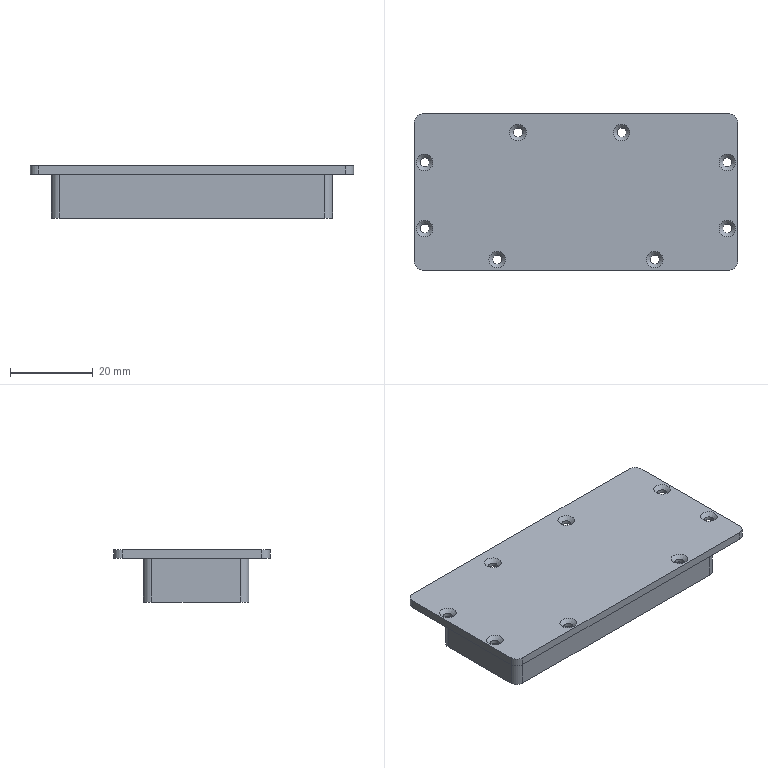Part | STEP file | 2-in-1 cover | 1 solid | 59 faces | box 78 x 37.65 x 12.6 mm | volume 23932 mm3 | cylinder 24 | plane 19 | cone 16 | commonest cylinder face diameters 2.1 x8 2.2 x8 4 x8